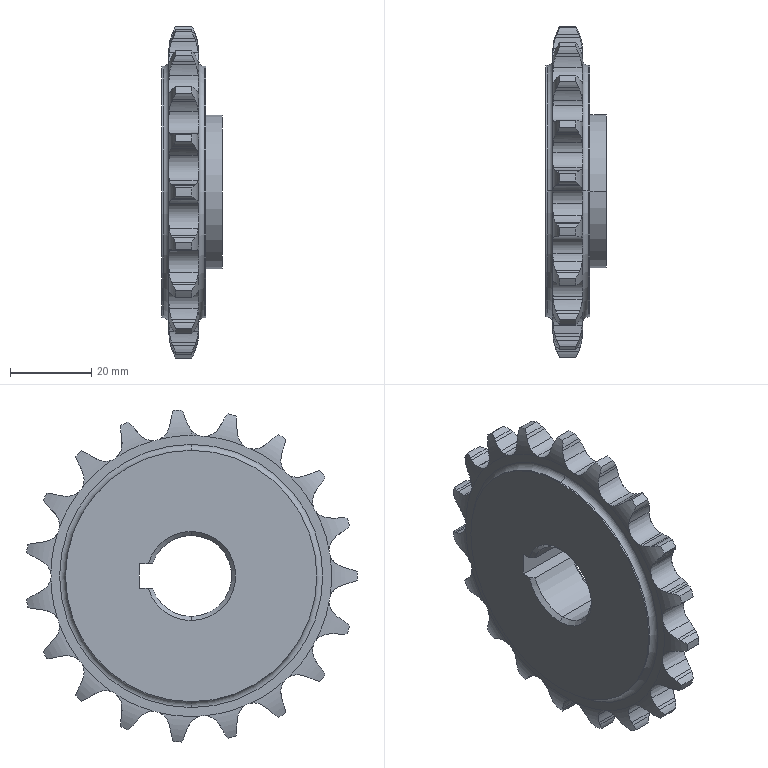Part | SolidWorks | features Chamfer 2, Cut 2, Revolution 2, CirPattern 1 | 1 solid | 228 faces | box 15 x 81.595 x 81.862 mm | volume 41818 mm3 | cylinder 132 | plane 46 | torus 44 | cone 6 | commonest cylinder face diameters 11.518 x40 20.732 x40 8.06 x24 82 x19 62 x4 20 x3